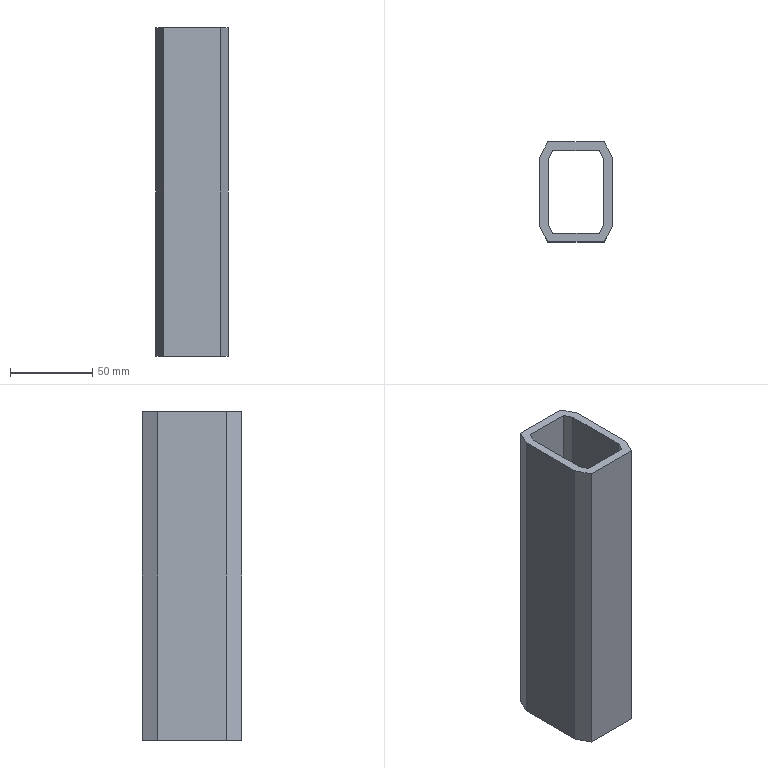Part | SolidWorks | features Extrusion 1 | 1 solid | 18 faces | box 44 x 60.7 x 200 mm | volume 178016 mm3 | plane 18
STEP:
#1=CARTESIAN_POINT('',(-17.32,136.5,200.));
#2=VERTEX_POINT('',#1);
#3=CARTESIAN_POINT('',(-22.,127.139,200.));
#4=VERTEX_POINT('',#3);
#5=CARTESIAN_POINT('',(-22.,127.139,200.));
#6=DIRECTION('',(-0.4472,-0.8944,0.));
#7=VECTOR('',#6,1000.);
#8=LINE('',#5,#7);
#9=EDGE_CURVE('',#2,#4,#8,.T.);
#10=ORIENTED_EDGE('',*,*,#9,.T.);
#11=CARTESIAN_POINT('',(-22.,85.161,200.));
#12=VERTEX_POINT('',#11);
#13=CARTESIAN_POINT('',(-22.,85.161,200.));
#14=DIRECTION('',(0.,-1.,0.));
#15=VECTOR('',#14,1000.);
#16=LINE('',#13,#15);
#17=EDGE_CURVE('',#4,#12,#16,.T.);
#18=ORIENTED_EDGE('',*,*,#17,.T.);
#19=CARTESIAN_POINT('',(-17.32,75.8,200.));
#20=VERTEX_POINT('',#19);
#21=CARTESIAN_POINT('',(-17.32,75.8,200.));
#22=DIRECTION('',(0.4472,-0.8944,0.));
#23=VECTOR('',#22,1000.);
#24=LINE('',#21,#23);
#25=EDGE_CURVE('',#12,#20,#24,.T.);
#26=ORIENTED_EDGE('',*,*,#25,.T.);
#27=CARTESIAN_POINT('',(17.32,75.8,200.));
#28=VERTEX_POINT('',#27);
#29=CARTESIAN_POINT('',(17.32,75.8,200.));
#30=DIRECTION('',(1.,0.,0.));
#31=VECTOR('',#30,1000.);
#32=LINE('',#29,#31);
#33=EDGE_CURVE('',#20,#28,#32,.T.);
#34=ORIENTED_EDGE('',*,*,#33,.T.);
#35=CARTESIAN_POINT('',(22.,85.161,200.));
#36=VERTEX_POINT('',#35);
#37=CARTESIAN_POINT('',(22.,85.161,200.));
#38=DIRECTION('',(0.4472,0.8944,0.));
#39=VECTOR('',#38,1000.);
#40=LINE('',#37,#39);
#41=EDGE_CURVE('',#28,#36,#40,.T.);
#42=ORIENTED_EDGE('',*,*,#41,.T.);
#43=CARTESIAN_POINT('',(22.,127.139,200.));
#44=VERTEX_POINT('',#43);
#45=CARTESIAN_POINT('',(22.,127.139,200.));
#46=DIRECTION('',(0.,1.,0.));
#47=VECTOR('',#46,1000.);
#48=LINE('',#45,#47);
#49=EDGE_CURVE('',#36,#44,#48,.T.);
#50=ORIENTED_EDGE('',*,*,#49,.T.);
#51=CARTESIAN_POINT('',(17.32,136.5,200.));
#52=VERTEX_POINT('',#51);
#53=CARTESIAN_POINT('',(17.32,136.5,200.));
#54=DIRECTION('',(-0.4472,0.8944,0.));
#55=VECTOR('',#54,1000.);
#56=LINE('',#53,#55);
#57=EDGE_CURVE('',#44,#52,#56,.T.);
#58=ORIENTED_EDGE('',*,*,#57,.T.);
#59=CARTESIAN_POINT('',(-17.32,136.5,200.));
#60=DIRECTION('',(-1.,0.,0.));
#61=VECTOR('',#60,1000.);
#62=LINE('',#59,#61);
#63=EDGE_CURVE('',#52,#2,#62,.T.);
#64=ORIENTED_EDGE('',*,*,#63,.T.);
#65=EDGE_LOOP('',(#10,#18,#26,#34,#42,#50,#58,#64));
#66=FACE_OUTER_BOUND('',#65,.T.);
#67=CARTESIAN_POINT('',(-14.229,131.5,200.));
#68=VERTEX_POINT('',#67);
#69=CARTESIAN_POINT('',(-17.,125.959,200.));
#70=VERTEX_POINT('',#69);
#71=CARTESIAN_POINT('',(-17.,125.959,200.));
#72=DIRECTION('',(-0.4472,-0.8944,0.));
#73=VECTOR('',#72,1000.);
#74=LINE('',#71,#73);
#75=EDGE_CURVE('',#68,#70,#74,.T.);
#76=ORIENTED_EDGE('',*,*,#75,.F.);
#77=CARTESIAN_POINT('',(14.229,131.5,200.));
#78=VERTEX_POINT('',#77);
#79=CARTESIAN_POINT('',(-14.229,131.5,200.));
#80=DIRECTION('',(-1.,0.,0.));
#81=VECTOR('',#80,1000.);
#82=LINE('',#79,#81);
#83=EDGE_CURVE('',#78,#68,#82,.T.);
#84=ORIENTED_EDGE('',*,*,#83,.F.);
#85=CARTESIAN_POINT('',(17.,125.959,200.));
#86=VERTEX_POINT('',#85);
#87=CARTESIAN_POINT('',(14.229,131.5,200.));
#88=DIRECTION('',(-0.4472,0.8944,0.));
#89=VECTOR('',#88,1000.);
#90=LINE('',#87,#89);
#91=EDGE_CURVE('',#86,#78,#90,.T.);
#92=ORIENTED_EDGE('',*,*,#91,.F.);
#93=CARTESIAN_POINT('',(17.,86.341,200.));
#94=VERTEX_POINT('',#93);
#95=CARTESIAN_POINT('',(17.,125.959,200.));
#96=DIRECTION('',(0.,1.,0.));
#97=VECTOR('',#96,1000.);
#98=LINE('',#95,#97);
#99=EDGE_CURVE('',#94,#86,#98,.T.);
#100=ORIENTED_EDGE('',*,*,#99,.F.);
#101=CARTESIAN_POINT('',(14.229,80.8,200.));
#102=VERTEX_POINT('',#101);
#103=CARTESIAN_POINT('',(17.,86.341,200.));
#104=DIRECTION('',(0.4472,0.8944,0.));
#105=VECTOR('',#104,1000.);
#106=LINE('',#103,#105);
#107=EDGE_CURVE('',#102,#94,#106,.T.);
#108=ORIENTED_EDGE('',*,*,#107,.F.);
#109=CARTESIAN_POINT('',(-14.229,80.8,200.));
#110=VERTEX_POINT('',#109);
#111=CARTESIAN_POINT('',(14.229,80.8,200.));
#112=DIRECTION('',(1.,0.,0.));
#113=VECTOR('',#112,1000.);
#114=LINE('',#111,#113);
#115=EDGE_CURVE('',#110,#102,#114,.T.);
#116=ORIENTED_EDGE('',*,*,#115,.F.);
#117=CARTESIAN_POINT('',(-17.,86.341,200.));
#118=VERTEX_POINT('',#117);
#119=CARTESIAN_POINT('',(-14.229,80.8,200.));
#120=DIRECTION('',(0.4472,-0.8944,0.));
#121=VECTOR('',#120,1000.);
#122=LINE('',#119,#121);
#123=EDGE_CURVE('',#118,#110,#122,.T.);
#124=ORIENTED_EDGE('',*,*,#123,.F.);
#125=CARTESIAN_POINT('',(-17.,86.341,200.));
#126=DIRECTION('',(0.,-1.,0.));
#127=VECTOR('',#126,1000.);
#128=LINE('',#125,#127);
#129=EDGE_CURVE('',#70,#118,#128,.T.);
#130=ORIENTED_EDGE('',*,*,#129,.F.);
#131=EDGE_LOOP('',(#76,#84,#92,#100,#108,#116,#124,#130));
#132=FACE_BOUND('',#131,.T.);
#133=CARTESIAN_POINT('',(0.,0.,200.));
#134=DIRECTION('',(0.,0.,-1.));
#135=DIRECTION('',(-1.,0.,0.));
#136=AXIS2_PLACEMENT_3D('',#133,#134,#135);
#137=PLANE('',#136);
#138=ADVANCED_FACE('',(#66,#132),#137,.F.);
#139=CARTESIAN_POINT('',(-17.32,136.5,0.));
#140=VERTEX_POINT('',#139);
#141=CARTESIAN_POINT('',(-22.,127.139,0.));
#142=VERTEX_POINT('',#141);
#143=CARTESIAN_POINT('',(-22.,127.139,0.));
#144=DIRECTION('',(-0.4472,-0.8944,0.));
#145=VECTOR('',#144,1000.);
#146=LINE('',#143,#145);
#147=EDGE_CURVE('',#140,#142,#146,.T.);
#148=ORIENTED_EDGE('',*,*,#147,.F.);
#149=CARTESIAN_POINT('',(17.32,136.5,0.));
#150=VERTEX_POINT('',#149);
#151=CARTESIAN_POINT('',(-17.32,136.5,0.));
#152=DIRECTION('',(-1.,0.,0.));
#153=VECTOR('',#152,1000.);
#154=LINE('',#151,#153);
#155=EDGE_CURVE('',#150,#140,#154,.T.);
#156=ORIENTED_EDGE('',*,*,#155,.F.);
#157=CARTESIAN_POINT('',(22.,127.139,0.));
#158=VERTEX_POINT('',#157);
#159=CARTESIAN_POINT('',(17.32,136.5,0.));
#160=DIRECTION('',(-0.4472,0.8944,0.));
#161=VECTOR('',#160,1000.);
#162=LINE('',#159,#161);
#163=EDGE_CURVE('',#158,#150,#162,.T.);
#164=ORIENTED_EDGE('',*,*,#163,.F.);
#165=CARTESIAN_POINT('',(22.,85.161,0.));
#166=VERTEX_POINT('',#165);
#167=CARTESIAN_POINT('',(22.,127.139,0.));
#168=DIRECTION('',(0.,1.,0.));
#169=VECTOR('',#168,1000.);
#170=LINE('',#167,#169);
#171=EDGE_CURVE('',#166,#158,#170,.T.);
#172=ORIENTED_EDGE('',*,*,#171,.F.);
#173=CARTESIAN_POINT('',(17.32,75.8,0.));
#174=VERTEX_POINT('',#173);
#175=CARTESIAN_POINT('',(22.,85.161,0.));
#176=DIRECTION('',(0.4472,0.8944,0.));
#177=VECTOR('',#176,1000.);
#178=LINE('',#175,#177);
#179=EDGE_CURVE('',#174,#166,#178,.T.);
#180=ORIENTED_EDGE('',*,*,#179,.F.);
#181=CARTESIAN_POINT('',(-17.32,75.8,0.));
#182=VERTEX_POINT('',#181);
#183=CARTESIAN_POINT('',(17.32,75.8,0.));
#184=DIRECTION('',(1.,0.,0.));
#185=VECTOR('',#184,1000.);
#186=LINE('',#183,#185);
#187=EDGE_CURVE('',#182,#174,#186,.T.);
#188=ORIENTED_EDGE('',*,*,#187,.F.);
#189=CARTESIAN_POINT('',(-22.,85.161,0.));
#190=VERTEX_POINT('',#189);
#191=CARTESIAN_POINT('',(-17.32,75.8,0.));
#192=DIRECTION('',(0.4472,-0.8944,0.));
#193=VECTOR('',#192,1000.);
#194=LINE('',#191,#193);
#195=EDGE_CURVE('',#190,#182,#194,.T.);
#196=ORIENTED_EDGE('',*,*,#195,.F.);
#197=CARTESIAN_POINT('',(-22.,85.161,0.));
#198=DIRECTION('',(0.,-1.,0.));
#199=VECTOR('',#198,1000.);
#200=LINE('',#197,#199);
#201=EDGE_CURVE('',#142,#190,#200,.T.);
#202=ORIENTED_EDGE('',*,*,#201,.F.);
#203=EDGE_LOOP('',(#148,#156,#164,#172,#180,#188,#196,#202));
#204=FACE_OUTER_BOUND('',#203,.T.);
#205=CARTESIAN_POINT('',(14.229,131.5,0.));
#206=VERTEX_POINT('',#205);
#207=CARTESIAN_POINT('',(-14.229,131.5,0.));
#208=VERTEX_POINT('',#207);
#209=CARTESIAN_POINT('',(-14.229,131.5,0.));
#210=DIRECTION('',(-1.,0.,0.));
#211=VECTOR('',#210,1000.);
#212=LINE('',#209,#211);
#213=EDGE_CURVE('',#206,#208,#212,.T.);
#214=ORIENTED_EDGE('',*,*,#213,.T.);
#215=CARTESIAN_POINT('',(-17.,125.959,0.));
#216=VERTEX_POINT('',#215);
#217=CARTESIAN_POINT('',(-17.,125.959,0.));
#218=DIRECTION('',(-0.4472,-0.8944,0.));
#219=VECTOR('',#218,1000.);
#220=LINE('',#217,#219);
#221=EDGE_CURVE('',#208,#216,#220,.T.);
#222=ORIENTED_EDGE('',*,*,#221,.T.);
#223=CARTESIAN_POINT('',(-17.,86.341,0.));
#224=VERTEX_POINT('',#223);
#225=CARTESIAN_POINT('',(-17.,86.341,0.));
#226=DIRECTION('',(0.,-1.,0.));
#227=VECTOR('',#226,1000.);
#228=LINE('',#225,#227);
#229=EDGE_CURVE('',#216,#224,#228,.T.);
#230=ORIENTED_EDGE('',*,*,#229,.T.);
#231=CARTESIAN_POINT('',(-14.229,80.8,0.));
#232=VERTEX_POINT('',#231);
#233=CARTESIAN_POINT('',(-14.229,80.8,0.));
#234=DIRECTION('',(0.4472,-0.8944,0.));
#235=VECTOR('',#234,1000.);
#236=LINE('',#233,#235);
#237=EDGE_CURVE('',#224,#232,#236,.T.);
#238=ORIENTED_EDGE('',*,*,#237,.T.);
#239=CARTESIAN_POINT('',(14.229,80.8,0.));
#240=VERTEX_POINT('',#239);
#241=CARTESIAN_POINT('',(14.229,80.8,0.));
#242=DIRECTION('',(1.,0.,0.));
#243=VECTOR('',#242,1000.);
#244=LINE('',#241,#243);
#245=EDGE_CURVE('',#232,#240,#244,.T.);
#246=ORIENTED_EDGE('',*,*,#245,.T.);
#247=CARTESIAN_POINT('',(17.,86.341,0.));
#248=VERTEX_POINT('',#247);
#249=CARTESIAN_POINT('',(17.,86.341,0.));
#250=DIRECTION('',(0.4472,0.8944,0.));
#251=VECTOR('',#250,1000.);
#252=LINE('',#249,#251);
#253=EDGE_CURVE('',#240,#248,#252,.T.);
#254=ORIENTED_EDGE('',*,*,#253,.T.);
#255=CARTESIAN_POINT('',(17.,125.959,0.));
#256=VERTEX_POINT('',#255);
#257=CARTESIAN_POINT('',(17.,125.959,0.));
#258=DIRECTION('',(0.,1.,0.));
#259=VECTOR('',#258,1000.);
#260=LINE('',#257,#259);
#261=EDGE_CURVE('',#248,#256,#260,.T.);
#262=ORIENTED_EDGE('',*,*,#261,.T.);
#263=CARTESIAN_POINT('',(14.229,131.5,0.));
#264=DIRECTION('',(-0.4472,0.8944,0.));
#265=VECTOR('',#264,1000.);
#266=LINE('',#263,#265);
#267=EDGE_CURVE('',#256,#206,#266,.T.);
#268=ORIENTED_EDGE('',*,*,#267,.T.);
#269=EDGE_LOOP('',(#214,#222,#230,#238,#246,#254,#262,#268));
#270=FACE_BOUND('',#269,.T.);
#271=CARTESIAN_POINT('',(0.,0.,0.));
#272=DIRECTION('',(0.,0.,-1.));
#273=DIRECTION('',(-1.,0.,0.));
#274=AXIS2_PLACEMENT_3D('',#271,#272,#273);
#275=PLANE('',#274);
#276=ADVANCED_FACE('',(#204,#270),#275,.T.);
#277=ORIENTED_EDGE('',*,*,#147,.T.);
#278=CARTESIAN_POINT('',(-22.,127.139,200.));
#279=DIRECTION('',(0.,0.,-1.));
#280=VECTOR('',#279,1000.);
#281=LINE('',#278,#280);
#282=EDGE_CURVE('',#4,#142,#281,.T.);
#283=ORIENTED_EDGE('',*,*,#282,.F.);
#284=ORIENTED_EDGE('',*,*,#9,.F.);
#285=CARTESIAN_POINT('',(-17.32,136.5,200.));
#286=DIRECTION('',(0.,0.,-1.));
#287=VECTOR('',#286,1000.);
#288=LINE('',#285,#287);
#289=EDGE_CURVE('',#2,#140,#288,.T.);
#290=ORIENTED_EDGE('',*,*,#289,.T.);
#291=EDGE_LOOP('',(#277,#283,#284,#290));
#292=FACE_OUTER_BOUND('',#291,.T.);
#293=CARTESIAN_POINT('',(-22.,127.139,200.));
#294=DIRECTION('',(0.8944,-0.4472,0.));
#295=DIRECTION('',(0.4472,0.8944,0.));
#296=AXIS2_PLACEMENT_3D('',#293,#294,#295);
#297=PLANE('',#296);
#298=ADVANCED_FACE('',(#292),#297,.F.);
#299=ORIENTED_EDGE('',*,*,#201,.T.);
#300=CARTESIAN_POINT('',(-22.,85.161,200.));
#301=DIRECTION('',(0.,0.,-1.));
#302=VECTOR('',#301,1000.);
#303=LINE('',#300,#302);
#304=EDGE_CURVE('',#12,#190,#303,.T.);
#305=ORIENTED_EDGE('',*,*,#304,.F.);
#306=ORIENTED_EDGE('',*,*,#17,.F.);
#307=ORIENTED_EDGE('',*,*,#282,.T.);
#308=EDGE_LOOP('',(#299,#305,#306,#307));
#309=FACE_OUTER_BOUND('',#308,.T.);
#310=CARTESIAN_POINT('',(-22.,85.161,200.));
#311=DIRECTION('',(1.,0.,0.));
#312=DIRECTION('',(0.,1.,0.));
#313=AXIS2_PLACEMENT_3D('',#310,#311,#312);
#314=PLANE('',#313);
#315=ADVANCED_FACE('',(#309),#314,.F.);
#316=ORIENTED_EDGE('',*,*,#195,.T.);
#317=CARTESIAN_POINT('',(-17.32,75.8,200.));
#318=DIRECTION('',(0.,0.,-1.));
#319=VECTOR('',#318,1000.);
#320=LINE('',#317,#319);
#321=EDGE_CURVE('',#20,#182,#320,.T.);
#322=ORIENTED_EDGE('',*,*,#321,.F.);
#323=ORIENTED_EDGE('',*,*,#25,.F.);
#324=ORIENTED_EDGE('',*,*,#304,.T.);
#325=EDGE_LOOP('',(#316,#322,#323,#324));
#326=FACE_OUTER_BOUND('',#325,.T.);
#327=CARTESIAN_POINT('',(-17.32,75.8,200.));
#328=DIRECTION('',(0.8944,0.4472,0.));
#329=DIRECTION('',(-0.4472,0.8944,0.));
#330=AXIS2_PLACEMENT_3D('',#327,#328,#329);
#331=PLANE('',#330);
#332=ADVANCED_FACE('',(#326),#331,.F.);
#333=ORIENTED_EDGE('',*,*,#187,.T.);
#334=CARTESIAN_POINT('',(17.32,75.8,200.));
#335=DIRECTION('',(0.,0.,-1.));
#336=VECTOR('',#335,1000.);
#337=LINE('',#334,#336);
#338=EDGE_CURVE('',#28,#174,#337,.T.);
#339=ORIENTED_EDGE('',*,*,#338,.F.);
#340=ORIENTED_EDGE('',*,*,#33,.F.);
#341=ORIENTED_EDGE('',*,*,#321,.T.);
#342=EDGE_LOOP('',(#333,#339,#340,#341));
#343=FACE_OUTER_BOUND('',#342,.T.);
#344=CARTESIAN_POINT('',(17.32,75.8,200.));
#345=DIRECTION('',(0.,1.,0.));
#346=DIRECTION('',(-1.,0.,0.));
#347=AXIS2_PLACEMENT_3D('',#344,#345,#346);
#348=PLANE('',#347);
#349=ADVANCED_FACE('',(#343),#348,.F.);
#350=ORIENTED_EDGE('',*,*,#179,.T.);
#351=CARTESIAN_POINT('',(22.,85.161,200.));
#352=DIRECTION('',(0.,0.,-1.));
#353=VECTOR('',#352,1000.);
#354=LINE('',#351,#353);
#355=EDGE_CURVE('',#36,#166,#354,.T.);
#356=ORIENTED_EDGE('',*,*,#355,.F.);
#357=ORIENTED_EDGE('',*,*,#41,.F.);
#358=ORIENTED_EDGE('',*,*,#338,.T.);
#359=EDGE_LOOP('',(#350,#356,#357,#358));
#360=FACE_OUTER_BOUND('',#359,.T.);
#361=CARTESIAN_POINT('',(22.,85.161,200.));
#362=DIRECTION('',(-0.8944,0.4472,0.));
#363=DIRECTION('',(-0.4472,-0.8944,0.));
#364=AXIS2_PLACEMENT_3D('',#361,#362,#363);
#365=PLANE('',#364);
#366=ADVANCED_FACE('',(#360),#365,.F.);
#367=ORIENTED_EDGE('',*,*,#171,.T.);
#368=CARTESIAN_POINT('',(22.,127.139,200.));
#369=DIRECTION('',(0.,0.,-1.));
#370=VECTOR('',#369,1000.);
#371=LINE('',#368,#370);
#372=EDGE_CURVE('',#44,#158,#371,.T.);
#373=ORIENTED_EDGE('',*,*,#372,.F.);
#374=ORIENTED_EDGE('',*,*,#49,.F.);
#375=ORIENTED_EDGE('',*,*,#355,.T.);
#376=EDGE_LOOP('',(#367,#373,#374,#375));
#377=FACE_OUTER_BOUND('',#376,.T.);
#378=CARTESIAN_POINT('',(22.,127.139,200.));
#379=DIRECTION('',(-1.,0.,0.));
#380=DIRECTION('',(0.,-1.,0.));
#381=AXIS2_PLACEMENT_3D('',#378,#379,#380);
#382=PLANE('',#381);
#383=ADVANCED_FACE('',(#377),#382,.F.);
#384=ORIENTED_EDGE('',*,*,#163,.T.);
#385=CARTESIAN_POINT('',(17.32,136.5,200.));
#386=DIRECTION('',(0.,0.,-1.));
#387=VECTOR('',#386,1000.);
#388=LINE('',#385,#387);
#389=EDGE_CURVE('',#52,#150,#388,.T.);
#390=ORIENTED_EDGE('',*,*,#389,.F.);
#391=ORIENTED_EDGE('',*,*,#57,.F.);
#392=ORIENTED_EDGE('',*,*,#372,.T.);
#393=EDGE_LOOP('',(#384,#390,#391,#392));
#394=FACE_OUTER_BOUND('',#393,.T.);
#395=CARTESIAN_POINT('',(17.32,136.5,200.));
#396=DIRECTION('',(-0.8944,-0.4472,0.));
#397=DIRECTION('',(0.4472,-0.8944,0.));
#398=AXIS2_PLACEMENT_3D('',#395,#396,#397);
#399=PLANE('',#398);
#400=ADVANCED_FACE('',(#394),#399,.F.);
#401=ORIENTED_EDGE('',*,*,#155,.T.);
#402=ORIENTED_EDGE('',*,*,#289,.F.);
#403=ORIENTED_EDGE('',*,*,#63,.F.);
#404=ORIENTED_EDGE('',*,*,#389,.T.);
#405=EDGE_LOOP('',(#401,#402,#403,#404));
#406=FACE_OUTER_BOUND('',#405,.T.);
#407=CARTESIAN_POINT('',(-17.32,136.5,200.));
#408=DIRECTION('',(0.,-1.,0.));
#409=DIRECTION('',(0.,0.,-1.));
#410=AXIS2_PLACEMENT_3D('',#407,#408,#409);
#411=PLANE('',#410);
#412=ADVANCED_FACE('',(#406),#411,.F.);
#413=ORIENTED_EDGE('',*,*,#221,.F.);
#414=CARTESIAN_POINT('',(-14.229,131.5,200.));
#415=DIRECTION('',(0.,0.,-1.));
#416=VECTOR('',#415,1000.);
#417=LINE('',#414,#416);
#418=EDGE_CURVE('',#68,#208,#417,.T.);
#419=ORIENTED_EDGE('',*,*,#418,.F.);
#420=ORIENTED_EDGE('',*,*,#75,.T.);
#421=CARTESIAN_POINT('',(-17.,125.959,200.));
#422=DIRECTION('',(0.,0.,-1.));
#423=VECTOR('',#422,1000.);
#424=LINE('',#421,#423);
#425=EDGE_CURVE('',#70,#216,#424,.T.);
#426=ORIENTED_EDGE('',*,*,#425,.T.);
#427=EDGE_LOOP('',(#413,#419,#420,#426));
#428=FACE_OUTER_BOUND('',#427,.T.);
#429=CARTESIAN_POINT('',(-17.,125.959,200.));
#430=DIRECTION('',(0.8944,-0.4472,0.));
#431=DIRECTION('',(0.4472,0.8944,0.));
#432=AXIS2_PLACEMENT_3D('',#429,#430,#431);
#433=PLANE('',#432);
#434=ADVANCED_FACE('',(#428),#433,.T.);
#435=ORIENTED_EDGE('',*,*,#229,.F.);
#436=ORIENTED_EDGE('',*,*,#425,.F.);
#437=ORIENTED_EDGE('',*,*,#129,.T.);
#438=CARTESIAN_POINT('',(-17.,86.341,200.));
#439=DIRECTION('',(0.,0.,-1.));
#440=VECTOR('',#439,1000.);
#441=LINE('',#438,#440);
#442=EDGE_CURVE('',#118,#224,#441,.T.);
#443=ORIENTED_EDGE('',*,*,#442,.T.);
#444=EDGE_LOOP('',(#435,#436,#437,#443));
#445=FACE_OUTER_BOUND('',#444,.T.);
#446=CARTESIAN_POINT('',(-17.,86.341,200.));
#447=DIRECTION('',(1.,0.,0.));
#448=DIRECTION('',(0.,0.,-1.));
#449=AXIS2_PLACEMENT_3D('',#446,#447,#448);
#450=PLANE('',#449);
#451=ADVANCED_FACE('',(#445),#450,.T.);
#452=ORIENTED_EDGE('',*,*,#237,.F.);
#453=ORIENTED_EDGE('',*,*,#442,.F.);
#454=ORIENTED_EDGE('',*,*,#123,.T.);
#455=CARTESIAN_POINT('',(-14.229,80.8,200.));
#456=DIRECTION('',(0.,0.,-1.));
#457=VECTOR('',#456,1000.);
#458=LINE('',#455,#457);
#459=EDGE_CURVE('',#110,#232,#458,.T.);
#460=ORIENTED_EDGE('',*,*,#459,.T.);
#461=EDGE_LOOP('',(#452,#453,#454,#460));
#462=FACE_OUTER_BOUND('',#461,.T.);
#463=CARTESIAN_POINT('',(-14.229,80.8,200.));
#464=DIRECTION('',(0.8944,0.4472,0.));
#465=DIRECTION('',(-0.4472,0.8944,0.));
#466=AXIS2_PLACEMENT_3D('',#463,#464,#465);
#467=PLANE('',#466);
#468=ADVANCED_FACE('',(#462),#467,.T.);
#469=ORIENTED_EDGE('',*,*,#245,.F.);
#470=ORIENTED_EDGE('',*,*,#459,.F.);
#471=ORIENTED_EDGE('',*,*,#115,.T.);
#472=CARTESIAN_POINT('',(14.229,80.8,200.));
#473=DIRECTION('',(0.,0.,-1.));
#474=VECTOR('',#473,1000.);
#475=LINE('',#472,#474);
#476=EDGE_CURVE('',#102,#240,#475,.T.);
#477=ORIENTED_EDGE('',*,*,#476,.T.);
#478=EDGE_LOOP('',(#469,#470,#471,#477));
#479=FACE_OUTER_BOUND('',#478,.T.);
#480=CARTESIAN_POINT('',(14.229,80.8,200.));
#481=DIRECTION('',(0.,1.,0.));
#482=DIRECTION('',(0.,0.,1.));
#483=AXIS2_PLACEMENT_3D('',#480,#481,#482);
#484=PLANE('',#483);
#485=ADVANCED_FACE('',(#479),#484,.T.);
#486=ORIENTED_EDGE('',*,*,#253,.F.);
#487=ORIENTED_EDGE('',*,*,#476,.F.);
#488=ORIENTED_EDGE('',*,*,#107,.T.);
#489=CARTESIAN_POINT('',(17.,86.341,200.));
#490=DIRECTION('',(0.,0.,-1.));
#491=VECTOR('',#490,1000.);
#492=LINE('',#489,#491);
#493=EDGE_CURVE('',#94,#248,#492,.T.);
#494=ORIENTED_EDGE('',*,*,#493,.T.);
#495=EDGE_LOOP('',(#486,#487,#488,#494));
#496=FACE_OUTER_BOUND('',#495,.T.);
#497=CARTESIAN_POINT('',(17.,86.341,200.));
#498=DIRECTION('',(-0.8944,0.4472,0.));
#499=DIRECTION('',(-0.4472,-0.8944,0.));
#500=AXIS2_PLACEMENT_3D('',#497,#498,#499);
#501=PLANE('',#500);
#502=ADVANCED_FACE('',(#496),#501,.T.);
#503=ORIENTED_EDGE('',*,*,#261,.F.);
#504=ORIENTED_EDGE('',*,*,#493,.F.);
#505=ORIENTED_EDGE('',*,*,#99,.T.);
#506=CARTESIAN_POINT('',(17.,125.959,200.));
#507=DIRECTION('',(0.,0.,-1.));
#508=VECTOR('',#507,1000.);
#509=LINE('',#506,#508);
#510=EDGE_CURVE('',#86,#256,#509,.T.);
#511=ORIENTED_EDGE('',*,*,#510,.T.);
#512=EDGE_LOOP('',(#503,#504,#505,#511));
#513=FACE_OUTER_BOUND('',#512,.T.);
#514=CARTESIAN_POINT('',(17.,125.959,200.));
#515=DIRECTION('',(-1.,0.,0.));
#516=DIRECTION('',(0.,0.,1.));
#517=AXIS2_PLACEMENT_3D('',#514,#515,#516);
#518=PLANE('',#517);
#519=ADVANCED_FACE('',(#513),#518,.T.);
#520=ORIENTED_EDGE('',*,*,#267,.F.);
#521=ORIENTED_EDGE('',*,*,#510,.F.);
#522=ORIENTED_EDGE('',*,*,#91,.T.);
#523=CARTESIAN_POINT('',(14.229,131.5,200.));
#524=DIRECTION('',(0.,0.,-1.));
#525=VECTOR('',#524,1000.);
#526=LINE('',#523,#525);
#527=EDGE_CURVE('',#78,#206,#526,.T.);
#528=ORIENTED_EDGE('',*,*,#527,.T.);
#529=EDGE_LOOP('',(#520,#521,#522,#528));
#530=FACE_OUTER_BOUND('',#529,.T.);
#531=CARTESIAN_POINT('',(14.229,131.5,200.));
#532=DIRECTION('',(-0.8944,-0.4472,0.));
#533=DIRECTION('',(0.4472,-0.8944,0.));
#534=AXIS2_PLACEMENT_3D('',#531,#532,#533);
#535=PLANE('',#534);
#536=ADVANCED_FACE('',(#530),#535,.T.);
#537=ORIENTED_EDGE('',*,*,#213,.F.);
#538=ORIENTED_EDGE('',*,*,#527,.F.);
#539=ORIENTED_EDGE('',*,*,#83,.T.);
#540=ORIENTED_EDGE('',*,*,#418,.T.);
#541=EDGE_LOOP('',(#537,#538,#539,#540));
#542=FACE_OUTER_BOUND('',#541,.T.);
#543=CARTESIAN_POINT('',(-14.229,131.5,200.));
#544=DIRECTION('',(0.,-1.,0.));
#545=DIRECTION('',(0.,0.,-1.));
#546=AXIS2_PLACEMENT_3D('',#543,#544,#545);
#547=PLANE('',#546);
#548=ADVANCED_FACE('',(#542),#547,.T.);
#549=CLOSED_SHELL('',(#138,#276,#298,#315,#332,#349,#366,#383,#400,#412,#434,#451,#468,#485,#502,#519,#536,#548));
#550=MANIFOLD_SOLID_BREP('',#549);
#551=CARTESIAN_POINT('',(0.,0.,0.));
#552=DIRECTION('',(0.,0.,1.));
#553=DIRECTION('',(1.,0.,0.));
#554=AXIS2_PLACEMENT_3D('',#551,#552,#553);
#555=(LENGTH_UNIT()NAMED_UNIT(*)SI_UNIT(.MILLI.,.METRE.));
#556=UNCERTAINTY_MEASURE_WITH_UNIT(LENGTH_MEASURE(0.00001),#555,'','');
#557=(NAMED_UNIT(*)PLANE_ANGLE_UNIT()SI_UNIT($,.RADIAN.));
#558=(NAMED_UNIT(*)SI_UNIT($,.STERADIAN.)SOLID_ANGLE_UNIT());
#559=(GEOMETRIC_REPRESENTATION_CONTEXT(3)GLOBAL_UNCERTAINTY_ASSIGNED_CONTEXT((#556))GLOBAL_UNIT_ASSIGNED_CONTEXT((#555,#557,#558))REPRESENTATION_CONTEXT('',''));
#560=ADVANCED_BREP_SHAPE_REPRESENTATION('',(#550,#554),#559);